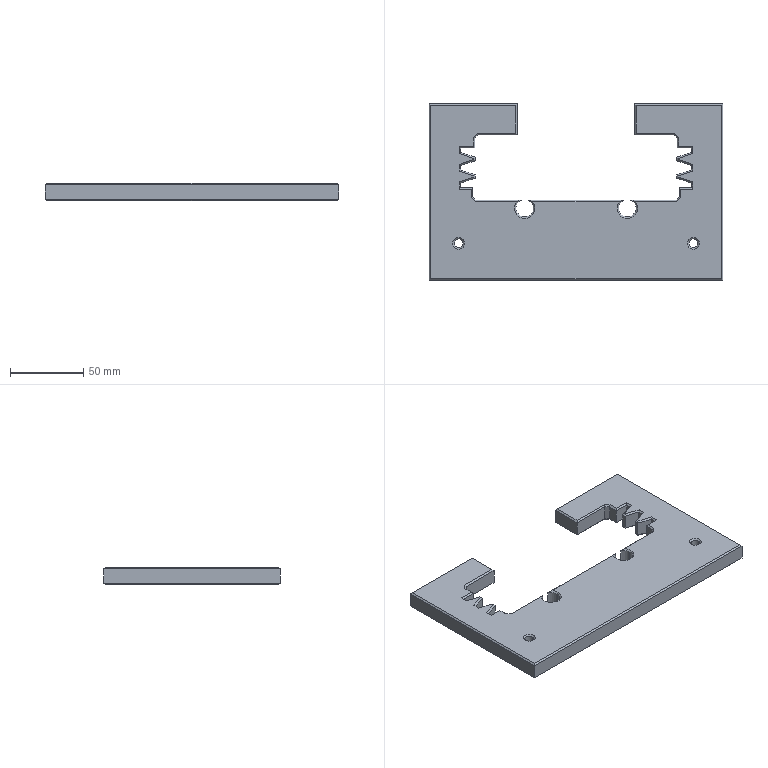Part | STEP file | Rotor mismatch gauge 2 | 1 solid | 301 faces | box 200 x 120 x 12 mm | volume 185907 mm3 | plane 223 | spline 51 | cone 17 | cylinder 10 | commonest cylinder face diameters 12 x6 6 x4